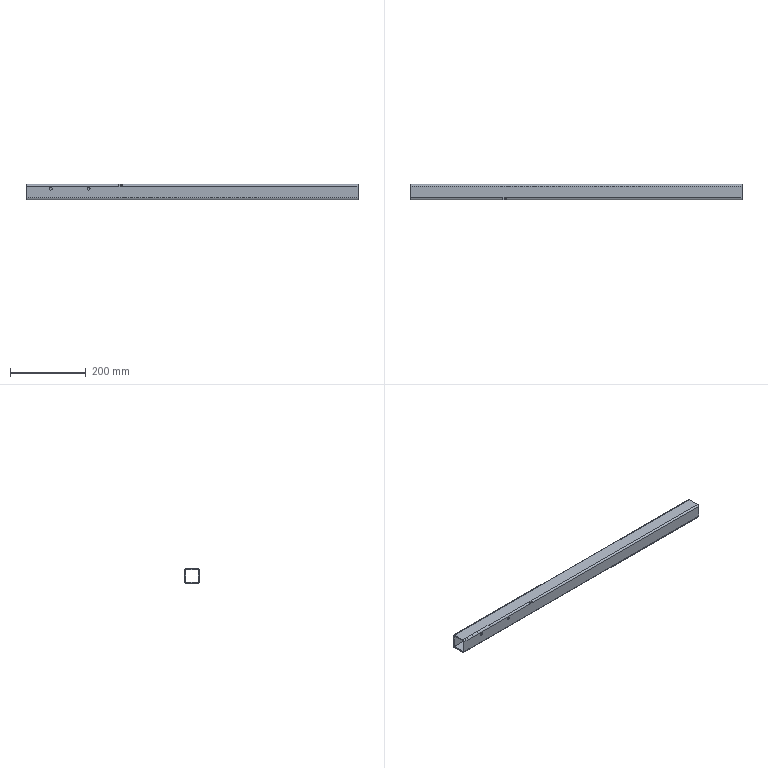Part | 1 solid | 23 faces | box 876 x 40 x 40 mm | volume 373261 mm3 | plane 14 | cylinder 9 | commonest cylinder face diameters 9 x5 8 x4
STEP:
#1=CARTESIAN_POINT('',(-373.,493.,624.88));
#2=VERTEX_POINT('',#1);
#3=CARTESIAN_POINT('',(-373.,493.,632.88));
#4=VERTEX_POINT('',#3);
#5=CARTESIAN_POINT('',(-373.,493.,628.88));
#6=DIRECTION('',(0.,1.,0.));
#7=DIRECTION('',(0.,0.,1.));
#8=AXIS2_PLACEMENT_3D('',#5,#6,#7);
#9=CIRCLE('',#8,4.);
#10=EDGE_CURVE('',#2,#4,#9,.T.);
#11=ORIENTED_EDGE('',*,*,#10,.T.);
#12=CARTESIAN_POINT('',(-373.,490.,632.88));
#13=VERTEX_POINT('',#12);
#14=CARTESIAN_POINT('',(-373.,490.,632.88));
#15=DIRECTION('',(0.,-1.,0.));
#16=VECTOR('',#15,1000.);
#17=LINE('',#14,#16);
#18=EDGE_CURVE('',#4,#13,#17,.T.);
#19=ORIENTED_EDGE('',*,*,#18,.T.);
#20=CARTESIAN_POINT('',(-373.,490.,624.88));
#21=VERTEX_POINT('',#20);
#22=CARTESIAN_POINT('',(-373.,490.,628.88));
#23=DIRECTION('',(0.,-1.,0.));
#24=DIRECTION('',(0.,0.,-1.));
#25=AXIS2_PLACEMENT_3D('',#22,#23,#24);
#26=CIRCLE('',#25,4.);
#27=EDGE_CURVE('',#13,#21,#26,.T.);
#28=ORIENTED_EDGE('',*,*,#27,.T.);
#29=CARTESIAN_POINT('',(-373.,490.,624.88));
#30=DIRECTION('',(0.,-1.,0.));
#31=VECTOR('',#30,1000.);
#32=LINE('',#29,#31);
#33=EDGE_CURVE('',#2,#21,#32,.T.);
#34=ORIENTED_EDGE('',*,*,#33,.F.);
#35=EDGE_LOOP('',(#11,#19,#28,#34));
#36=FACE_OUTER_BOUND('',#35,.T.);
#37=CARTESIAN_POINT('',(-373.,490.,628.88));
#38=DIRECTION('',(0.,-1.,0.));
#39=DIRECTION('',(0.,0.,-1.));
#40=AXIS2_PLACEMENT_3D('',#37,#38,#39);
#41=CYLINDRICAL_SURFACE('',#40,4.);
#42=ADVANCED_FACE('',(#36),#41,.F.);
#43=CARTESIAN_POINT('',(-473.,493.,624.88));
#44=VERTEX_POINT('',#43);
#45=CARTESIAN_POINT('',(-473.,493.,632.88));
#46=VERTEX_POINT('',#45);
#47=CARTESIAN_POINT('',(-473.,493.,628.88));
#48=DIRECTION('',(0.,1.,0.));
#49=DIRECTION('',(0.,0.,1.));
#50=AXIS2_PLACEMENT_3D('',#47,#48,#49);
#51=CIRCLE('',#50,4.);
#52=EDGE_CURVE('',#44,#46,#51,.T.);
#53=ORIENTED_EDGE('',*,*,#52,.T.);
#54=CARTESIAN_POINT('',(-473.,490.,632.88));
#55=VERTEX_POINT('',#54);
#56=CARTESIAN_POINT('',(-473.,490.,632.88));
#57=DIRECTION('',(0.,-1.,0.));
#58=VECTOR('',#57,1000.);
#59=LINE('',#56,#58);
#60=EDGE_CURVE('',#46,#55,#59,.T.);
#61=ORIENTED_EDGE('',*,*,#60,.T.);
#62=CARTESIAN_POINT('',(-473.,490.,624.88));
#63=VERTEX_POINT('',#62);
#64=CARTESIAN_POINT('',(-473.,490.,628.88));
#65=DIRECTION('',(0.,-1.,0.));
#66=DIRECTION('',(0.,0.,-1.));
#67=AXIS2_PLACEMENT_3D('',#64,#65,#66);
#68=CIRCLE('',#67,4.);
#69=EDGE_CURVE('',#55,#63,#68,.T.);
#70=ORIENTED_EDGE('',*,*,#69,.T.);
#71=CARTESIAN_POINT('',(-473.,490.,624.88));
#72=DIRECTION('',(0.,-1.,0.));
#73=VECTOR('',#72,1000.);
#74=LINE('',#71,#73);
#75=EDGE_CURVE('',#44,#63,#74,.T.);
#76=ORIENTED_EDGE('',*,*,#75,.F.);
#77=EDGE_LOOP('',(#53,#61,#70,#76));
#78=FACE_OUTER_BOUND('',#77,.T.);
#79=CARTESIAN_POINT('',(-473.,490.,628.88));
#80=DIRECTION('',(0.,-1.,0.));
#81=DIRECTION('',(0.,0.,-1.));
#82=AXIS2_PLACEMENT_3D('',#79,#80,#81);
#83=CYLINDRICAL_SURFACE('',#82,4.);
#84=ADVANCED_FACE('',(#78),#83,.F.);
#85=CARTESIAN_POINT('',(338.,525.5,640.));
#86=VERTEX_POINT('',#85);
#87=CARTESIAN_POINT('',(338.,494.5,640.));
#88=VERTEX_POINT('',#87);
#89=CARTESIAN_POINT('',(338.,530.,640.));
#90=DIRECTION('',(0.,-1.,0.));
#91=VECTOR('',#90,1000.);
#92=LINE('',#89,#91);
#93=EDGE_CURVE('',#86,#88,#92,.T.);
#94=ORIENTED_EDGE('',*,*,#93,.T.);
#95=CARTESIAN_POINT('',(338.,490.,635.5));
#96=VERTEX_POINT('',#95);
#97=CARTESIAN_POINT('',(338.,494.5,635.5));
#98=DIRECTION('',(1.,0.,0.));
#99=DIRECTION('',(0.,0.,1.));
#100=AXIS2_PLACEMENT_3D('',#97,#98,#99);
#101=CIRCLE('',#100,4.5);
#102=EDGE_CURVE('',#88,#96,#101,.T.);
#103=ORIENTED_EDGE('',*,*,#102,.T.);
#104=CARTESIAN_POINT('',(338.,490.,604.5));
#105=VERTEX_POINT('',#104);
#106=CARTESIAN_POINT('',(338.,490.,640.));
#107=DIRECTION('',(0.,0.,-1.));
#108=VECTOR('',#107,1000.);
#109=LINE('',#106,#108);
#110=EDGE_CURVE('',#96,#105,#109,.T.);
#111=ORIENTED_EDGE('',*,*,#110,.T.);
#112=CARTESIAN_POINT('',(338.,494.5,600.));
#113=VERTEX_POINT('',#112);
#114=CARTESIAN_POINT('',(338.,494.5,604.5));
#115=DIRECTION('',(1.,0.,0.));
#116=DIRECTION('',(0.,0.,1.));
#117=AXIS2_PLACEMENT_3D('',#114,#115,#116);
#118=CIRCLE('',#117,4.5);
#119=EDGE_CURVE('',#105,#113,#118,.T.);
#120=ORIENTED_EDGE('',*,*,#119,.T.);
#121=CARTESIAN_POINT('',(338.,525.5,600.));
#122=VERTEX_POINT('',#121);
#123=CARTESIAN_POINT('',(338.,490.,600.));
#124=DIRECTION('',(0.,-1.,0.));
#125=VECTOR('',#124,1000.);
#126=LINE('',#123,#125);
#127=EDGE_CURVE('',#122,#113,#126,.T.);
#128=ORIENTED_EDGE('',*,*,#127,.F.);
#129=CARTESIAN_POINT('',(338.,530.,604.5));
#130=VERTEX_POINT('',#129);
#131=CARTESIAN_POINT('',(338.,525.5,604.5));
#132=DIRECTION('',(1.,0.,0.));
#133=DIRECTION('',(0.,0.,1.));
#134=AXIS2_PLACEMENT_3D('',#131,#132,#133);
#135=CIRCLE('',#134,4.5);
#136=EDGE_CURVE('',#122,#130,#135,.T.);
#137=ORIENTED_EDGE('',*,*,#136,.T.);
#138=CARTESIAN_POINT('',(338.,530.,635.5));
#139=VERTEX_POINT('',#138);
#140=CARTESIAN_POINT('',(338.,530.,-260.));
#141=DIRECTION('',(0.,0.,-1.));
#142=VECTOR('',#141,1000.);
#143=LINE('',#140,#142);
#144=EDGE_CURVE('',#139,#130,#143,.T.);
#145=ORIENTED_EDGE('',*,*,#144,.F.);
#146=CARTESIAN_POINT('',(338.,525.5,635.5));
#147=DIRECTION('',(1.,0.,0.));
#148=DIRECTION('',(0.,0.,1.));
#149=AXIS2_PLACEMENT_3D('',#146,#147,#148);
#150=CIRCLE('',#149,4.5);
#151=EDGE_CURVE('',#139,#86,#150,.T.);
#152=ORIENTED_EDGE('',*,*,#151,.T.);
#153=EDGE_LOOP('',(#94,#103,#111,#120,#128,#137,#145,#152));
#154=FACE_OUTER_BOUND('',#153,.T.);
#155=CARTESIAN_POINT('',(338.,493.,637.));
#156=VERTEX_POINT('',#155);
#157=CARTESIAN_POINT('',(338.,493.,603.));
#158=VERTEX_POINT('',#157);
#159=CARTESIAN_POINT('',(338.,493.,-260.));
#160=DIRECTION('',(0.,0.,-1.));
#161=VECTOR('',#160,1000.);
#162=LINE('',#159,#161);
#163=EDGE_CURVE('',#156,#158,#162,.T.);
#164=ORIENTED_EDGE('',*,*,#163,.F.);
#165=CARTESIAN_POINT('',(338.,527.,637.));
#166=VERTEX_POINT('',#165);
#167=CARTESIAN_POINT('',(338.,490.,637.));
#168=DIRECTION('',(0.,-1.,0.));
#169=VECTOR('',#168,1000.);
#170=LINE('',#167,#169);
#171=EDGE_CURVE('',#166,#156,#170,.T.);
#172=ORIENTED_EDGE('',*,*,#171,.F.);
#173=CARTESIAN_POINT('',(338.,527.,603.));
#174=VERTEX_POINT('',#173);
#175=CARTESIAN_POINT('',(338.,527.,-260.));
#176=DIRECTION('',(0.,0.,1.));
#177=VECTOR('',#176,1000.);
#178=LINE('',#175,#177);
#179=EDGE_CURVE('',#174,#166,#178,.T.);
#180=ORIENTED_EDGE('',*,*,#179,.F.);
#181=CARTESIAN_POINT('',(338.,490.,603.));
#182=DIRECTION('',(0.,1.,0.));
#183=VECTOR('',#182,1000.);
#184=LINE('',#181,#183);
#185=EDGE_CURVE('',#158,#174,#184,.T.);
#186=ORIENTED_EDGE('',*,*,#185,.F.);
#187=EDGE_LOOP('',(#164,#172,#180,#186));
#188=FACE_BOUND('',#187,.T.);
#189=CARTESIAN_POINT('',(338.,490.,-260.));
#190=DIRECTION('',(-1.,0.,0.));
#191=DIRECTION('',(0.,0.,1.));
#192=AXIS2_PLACEMENT_3D('',#189,#190,#191);
#193=PLANE('',#192);
#194=ADVANCED_FACE('',(#154,#188),#193,.F.);
#195=CARTESIAN_POINT('',(-538.,494.5,640.));
#196=VERTEX_POINT('',#195);
#197=CARTESIAN_POINT('',(-538.,525.5,640.));
#198=VERTEX_POINT('',#197);
#199=CARTESIAN_POINT('',(-538.,530.,640.));
#200=DIRECTION('',(0.,1.,0.));
#201=VECTOR('',#200,1000.);
#202=LINE('',#199,#201);
#203=EDGE_CURVE('',#196,#198,#202,.T.);
#204=ORIENTED_EDGE('',*,*,#203,.T.);
#205=CARTESIAN_POINT('',(-538.,530.,635.5));
#206=VERTEX_POINT('',#205);
#207=CARTESIAN_POINT('',(-538.,525.5,635.5));
#208=DIRECTION('',(-1.,0.,0.));
#209=DIRECTION('',(0.,0.,-1.));
#210=AXIS2_PLACEMENT_3D('',#207,#208,#209);
#211=CIRCLE('',#210,4.5);
#212=EDGE_CURVE('',#198,#206,#211,.T.);
#213=ORIENTED_EDGE('',*,*,#212,.T.);
#214=CARTESIAN_POINT('',(-538.,530.,604.5));
#215=VERTEX_POINT('',#214);
#216=CARTESIAN_POINT('',(-538.,530.,640.));
#217=DIRECTION('',(0.,0.,1.));
#218=VECTOR('',#217,1000.);
#219=LINE('',#216,#218);
#220=EDGE_CURVE('',#215,#206,#219,.T.);
#221=ORIENTED_EDGE('',*,*,#220,.F.);
#222=CARTESIAN_POINT('',(-538.,525.5,600.));
#223=VERTEX_POINT('',#222);
#224=CARTESIAN_POINT('',(-538.,525.5,604.5));
#225=DIRECTION('',(-1.,0.,0.));
#226=DIRECTION('',(0.,0.,-1.));
#227=AXIS2_PLACEMENT_3D('',#224,#225,#226);
#228=CIRCLE('',#227,4.5);
#229=EDGE_CURVE('',#215,#223,#228,.T.);
#230=ORIENTED_EDGE('',*,*,#229,.T.);
#231=CARTESIAN_POINT('',(-538.,494.5,600.));
#232=VERTEX_POINT('',#231);
#233=CARTESIAN_POINT('',(-538.,490.,600.));
#234=DIRECTION('',(0.,1.,0.));
#235=VECTOR('',#234,1000.);
#236=LINE('',#233,#235);
#237=EDGE_CURVE('',#232,#223,#236,.T.);
#238=ORIENTED_EDGE('',*,*,#237,.F.);
#239=CARTESIAN_POINT('',(-538.,490.,604.5));
#240=VERTEX_POINT('',#239);
#241=CARTESIAN_POINT('',(-538.,494.5,604.5));
#242=DIRECTION('',(-1.,0.,0.));
#243=DIRECTION('',(0.,0.,-1.));
#244=AXIS2_PLACEMENT_3D('',#241,#242,#243);
#245=CIRCLE('',#244,4.5);
#246=EDGE_CURVE('',#232,#240,#245,.T.);
#247=ORIENTED_EDGE('',*,*,#246,.T.);
#248=CARTESIAN_POINT('',(-538.,490.,635.5));
#249=VERTEX_POINT('',#248);
#250=CARTESIAN_POINT('',(-538.,490.,640.));
#251=DIRECTION('',(0.,0.,-1.));
#252=VECTOR('',#251,1000.);
#253=LINE('',#250,#252);
#254=EDGE_CURVE('',#249,#240,#253,.T.);
#255=ORIENTED_EDGE('',*,*,#254,.F.);
#256=CARTESIAN_POINT('',(-538.,494.5,635.5));
#257=DIRECTION('',(-1.,0.,0.));
#258=DIRECTION('',(0.,0.,-1.));
#259=AXIS2_PLACEMENT_3D('',#256,#257,#258);
#260=CIRCLE('',#259,4.5);
#261=EDGE_CURVE('',#249,#196,#260,.T.);
#262=ORIENTED_EDGE('',*,*,#261,.T.);
#263=EDGE_LOOP('',(#204,#213,#221,#230,#238,#247,#255,#262));
#264=FACE_OUTER_BOUND('',#263,.T.);
#265=CARTESIAN_POINT('',(-538.,527.,637.));
#266=VERTEX_POINT('',#265);
#267=CARTESIAN_POINT('',(-538.,527.,603.));
#268=VERTEX_POINT('',#267);
#269=CARTESIAN_POINT('',(-538.,527.,640.));
#270=DIRECTION('',(0.,0.,-1.));
#271=VECTOR('',#270,1000.);
#272=LINE('',#269,#271);
#273=EDGE_CURVE('',#266,#268,#272,.T.);
#274=ORIENTED_EDGE('',*,*,#273,.F.);
#275=CARTESIAN_POINT('',(-538.,493.,637.));
#276=VERTEX_POINT('',#275);
#277=CARTESIAN_POINT('',(-538.,490.,637.));
#278=DIRECTION('',(0.,1.,0.));
#279=VECTOR('',#278,1000.);
#280=LINE('',#277,#279);
#281=EDGE_CURVE('',#276,#266,#280,.T.);
#282=ORIENTED_EDGE('',*,*,#281,.F.);
#283=CARTESIAN_POINT('',(-538.,493.,603.));
#284=VERTEX_POINT('',#283);
#285=CARTESIAN_POINT('',(-538.,493.,640.));
#286=DIRECTION('',(0.,0.,1.));
#287=VECTOR('',#286,1000.);
#288=LINE('',#285,#287);
#289=EDGE_CURVE('',#284,#276,#288,.T.);
#290=ORIENTED_EDGE('',*,*,#289,.F.);
#291=CARTESIAN_POINT('',(-538.,490.,603.));
#292=DIRECTION('',(0.,-1.,0.));
#293=VECTOR('',#292,1000.);
#294=LINE('',#291,#293);
#295=EDGE_CURVE('',#268,#284,#294,.T.);
#296=ORIENTED_EDGE('',*,*,#295,.F.);
#297=EDGE_LOOP('',(#274,#282,#290,#296));
#298=FACE_BOUND('',#297,.T.);
#299=CARTESIAN_POINT('',(-538.,490.,640.));
#300=DIRECTION('',(1.,0.,0.));
#301=DIRECTION('',(0.,0.,-1.));
#302=AXIS2_PLACEMENT_3D('',#299,#300,#301);
#303=PLANE('',#302);
#304=ADVANCED_FACE('',(#264,#298),#303,.F.);
#305=CARTESIAN_POINT('',(-293.2,494.5,640.));
#306=VERTEX_POINT('',#305);
#307=CARTESIAN_POINT('',(-293.2,490.,635.5));
#308=VERTEX_POINT('',#307);
#309=CARTESIAN_POINT('',(-293.2,494.5,635.5));
#310=DIRECTION('',(1.,0.,0.));
#311=DIRECTION('',(0.,0.,1.));
#312=AXIS2_PLACEMENT_3D('',#309,#310,#311);
#313=CIRCLE('',#312,4.5);
#314=EDGE_CURVE('',#306,#308,#313,.T.);
#315=ORIENTED_EDGE('',*,*,#314,.F.);
#316=CARTESIAN_POINT('',(160.,494.5,640.));
#317=DIRECTION('',(1.,0.,0.));
#318=VECTOR('',#317,1000.);
#319=LINE('',#316,#318);
#320=EDGE_CURVE('',#196,#306,#319,.T.);
#321=ORIENTED_EDGE('',*,*,#320,.F.);
#322=ORIENTED_EDGE('',*,*,#261,.F.);
#323=CARTESIAN_POINT('',(200.002,490.,635.5));
#324=DIRECTION('',(-1.,0.,0.));
#325=VECTOR('',#324,1000.);
#326=LINE('',#323,#325);
#327=EDGE_CURVE('',#308,#249,#326,.T.);
#328=ORIENTED_EDGE('',*,*,#327,.F.);
#329=EDGE_LOOP('',(#315,#321,#322,#328));
#330=FACE_OUTER_BOUND('',#329,.T.);
#331=CARTESIAN_POINT('',(200.002,494.5,635.5));
#332=DIRECTION('',(-1.,0.,0.));
#333=DIRECTION('',(0.,0.,1.));
#334=AXIS2_PLACEMENT_3D('',#331,#332,#333);
#335=CYLINDRICAL_SURFACE('',#334,4.5);
#336=ADVANCED_FACE('',(#330),#335,.T.);
#337=CARTESIAN_POINT('',(-373.,490.,628.88));
#338=DIRECTION('',(0.,-1.,0.));
#339=DIRECTION('',(0.,0.,-1.));
#340=AXIS2_PLACEMENT_3D('',#337,#338,#339);
#341=CIRCLE('',#340,4.);
#342=EDGE_CURVE('',#21,#13,#341,.T.);
#343=ORIENTED_EDGE('',*,*,#342,.F.);
#344=ORIENTED_EDGE('',*,*,#27,.F.);
#345=EDGE_LOOP('',(#343,#344));
#346=FACE_BOUND('',#345,.T.);
#347=CARTESIAN_POINT('',(-473.,490.,628.88));
#348=DIRECTION('',(0.,-1.,0.));
#349=DIRECTION('',(0.,0.,-1.));
#350=AXIS2_PLACEMENT_3D('',#347,#348,#349);
#351=CIRCLE('',#350,4.);
#352=EDGE_CURVE('',#63,#55,#351,.T.);
#353=ORIENTED_EDGE('',*,*,#352,.F.);
#354=ORIENTED_EDGE('',*,*,#69,.F.);
#355=EDGE_LOOP('',(#353,#354));
#356=FACE_BOUND('',#355,.T.);
#357=CARTESIAN_POINT('',(-293.2,490.,635.3));
#358=VERTEX_POINT('',#357);
#359=CARTESIAN_POINT('',(-282.8,490.,635.3));
#360=VERTEX_POINT('',#359);
#361=CARTESIAN_POINT('',(-293.2,490.,635.3));
#362=DIRECTION('',(1.,0.,0.));
#363=VECTOR('',#362,1000.);
#364=LINE('',#361,#363);
#365=EDGE_CURVE('',#358,#360,#364,.T.);
#366=ORIENTED_EDGE('',*,*,#365,.F.);
#367=CARTESIAN_POINT('',(-293.2,490.,635.3));
#368=DIRECTION('',(0.,0.,1.));
#369=VECTOR('',#368,1000.);
#370=LINE('',#367,#369);
#371=EDGE_CURVE('',#358,#308,#370,.T.);
#372=ORIENTED_EDGE('',*,*,#371,.T.);
#373=ORIENTED_EDGE('',*,*,#327,.T.);
#374=ORIENTED_EDGE('',*,*,#254,.T.);
#375=CARTESIAN_POINT('',(338.,490.,604.5));
#376=DIRECTION('',(1.,0.,0.));
#377=VECTOR('',#376,1000.);
#378=LINE('',#375,#377);
#379=EDGE_CURVE('',#240,#105,#378,.T.);
#380=ORIENTED_EDGE('',*,*,#379,.T.);
#381=ORIENTED_EDGE('',*,*,#110,.F.);
#382=CARTESIAN_POINT('',(-282.8,490.,635.5));
#383=VERTEX_POINT('',#382);
#384=CARTESIAN_POINT('',(200.002,490.,635.5));
#385=DIRECTION('',(-1.,0.,0.));
#386=VECTOR('',#385,1000.);
#387=LINE('',#384,#386);
#388=EDGE_CURVE('',#96,#383,#387,.T.);
#389=ORIENTED_EDGE('',*,*,#388,.T.);
#390=CARTESIAN_POINT('',(-282.8,490.,635.3));
#391=DIRECTION('',(0.,0.,1.));
#392=VECTOR('',#391,1000.);
#393=LINE('',#390,#392);
#394=EDGE_CURVE('',#360,#383,#393,.T.);
#395=ORIENTED_EDGE('',*,*,#394,.F.);
#396=EDGE_LOOP('',(#366,#372,#373,#374,#380,#381,#389,#395));
#397=FACE_OUTER_BOUND('',#396,.T.);
#398=CARTESIAN_POINT('',(200.002,490.,640.));
#399=DIRECTION('',(0.,1.,0.));
#400=DIRECTION('',(0.,0.,1.));
#401=AXIS2_PLACEMENT_3D('',#398,#399,#400);
#402=PLANE('',#401);
#403=ADVANCED_FACE('',(#346,#356,#397),#402,.F.);
#404=ORIENTED_EDGE('',*,*,#320,.T.);
#405=CARTESIAN_POINT('',(-293.2,494.7,640.));
#406=VERTEX_POINT('',#405);
#407=CARTESIAN_POINT('',(-293.2,494.7,640.));
#408=DIRECTION('',(0.,-1.,0.));
#409=VECTOR('',#408,1000.);
#410=LINE('',#407,#409);
#411=EDGE_CURVE('',#406,#306,#410,.T.);
#412=ORIENTED_EDGE('',*,*,#411,.F.);
#413=CARTESIAN_POINT('',(-282.8,494.7,640.));
#414=VERTEX_POINT('',#413);
#415=CARTESIAN_POINT('',(-282.8,494.7,640.));
#416=DIRECTION('',(-1.,0.,0.));
#417=VECTOR('',#416,1000.);
#418=LINE('',#415,#417);
#419=EDGE_CURVE('',#414,#406,#418,.T.);
#420=ORIENTED_EDGE('',*,*,#419,.F.);
#421=CARTESIAN_POINT('',(-282.8,494.5,640.));
#422=VERTEX_POINT('',#421);
#423=CARTESIAN_POINT('',(-282.8,490.,640.));
#424=DIRECTION('',(0.,1.,0.));
#425=VECTOR('',#424,1000.);
#426=LINE('',#423,#425);
#427=EDGE_CURVE('',#422,#414,#426,.T.);
#428=ORIENTED_EDGE('',*,*,#427,.F.);
#429=CARTESIAN_POINT('',(160.,494.5,640.));
#430=DIRECTION('',(1.,0.,0.));
#431=VECTOR('',#430,1000.);
#432=LINE('',#429,#431);
#433=EDGE_CURVE('',#422,#88,#432,.T.);
#434=ORIENTED_EDGE('',*,*,#433,.T.);
#435=ORIENTED_EDGE('',*,*,#93,.F.);
#436=CARTESIAN_POINT('',(160.,525.5,640.));
#437=DIRECTION('',(-1.,0.,0.));
#438=VECTOR('',#437,1000.);
#439=LINE('',#436,#438);
#440=EDGE_CURVE('',#86,#198,#439,.T.);
#441=ORIENTED_EDGE('',*,*,#440,.T.);
#442=ORIENTED_EDGE('',*,*,#203,.F.);
#443=EDGE_LOOP('',(#404,#412,#420,#428,#434,#435,#441,#442));
#444=FACE_OUTER_BOUND('',#443,.T.);
#445=CARTESIAN_POINT('',(160.,530.,640.));
#446=DIRECTION('',(0.,0.,-1.));
#447=DIRECTION('',(-1.,0.,0.));
#448=AXIS2_PLACEMENT_3D('',#445,#446,#447);
#449=PLANE('',#448);
#450=ADVANCED_FACE('',(#444),#449,.F.);
#451=ORIENTED_EDGE('',*,*,#220,.T.);
#452=CARTESIAN_POINT('',(200.,530.,635.5));
#453=DIRECTION('',(1.,0.,0.));
#454=VECTOR('',#453,1000.);
#455=LINE('',#452,#454);
#456=EDGE_CURVE('',#206,#139,#455,.T.);
#457=ORIENTED_EDGE('',*,*,#456,.T.);
#458=ORIENTED_EDGE('',*,*,#144,.T.);
#459=CARTESIAN_POINT('',(-538.,530.,604.5));
#460=DIRECTION('',(-1.,0.,0.));
#461=VECTOR('',#460,1000.);
#462=LINE('',#459,#461);
#463=EDGE_CURVE('',#130,#215,#462,.T.);
#464=ORIENTED_EDGE('',*,*,#463,.T.);
#465=EDGE_LOOP('',(#451,#457,#458,#464));
#466=FACE_OUTER_BOUND('',#465,.T.);
#467=CARTESIAN_POINT('',(200.,530.,-220.));
#468=DIRECTION('',(0.,-1.,0.));
#469=DIRECTION('',(0.,0.,-1.));
#470=AXIS2_PLACEMENT_3D('',#467,#468,#469);
#471=PLANE('',#470);
#472=ADVANCED_FACE('',(#466),#471,.F.);
#473=ORIENTED_EDGE('',*,*,#179,.T.);
#474=CARTESIAN_POINT('',(160.,527.,637.));
#475=DIRECTION('',(-1.,0.,0.));
#476=VECTOR('',#475,1000.);
#477=LINE('',#474,#476);
#478=EDGE_CURVE('',#166,#266,#477,.T.);
#479=ORIENTED_EDGE('',*,*,#478,.T.);
#480=ORIENTED_EDGE('',*,*,#273,.T.);
#481=CARTESIAN_POINT('',(-360.,527.,603.));
#482=DIRECTION('',(-1.,0.,0.));
#483=VECTOR('',#482,1000.);
#484=LINE('',#481,#483);
#485=EDGE_CURVE('',#174,#268,#484,.T.);
#486=ORIENTED_EDGE('',*,*,#485,.F.);
#487=EDGE_LOOP('',(#473,#479,#480,#486));
#488=FACE_OUTER_BOUND('',#487,.T.);
#489=CARTESIAN_POINT('',(-360.,527.,-330.));
#490=DIRECTION('',(0.,-1.,0.));
#491=DIRECTION('',(0.,0.,-1.));
#492=AXIS2_PLACEMENT_3D('',#489,#490,#491);
#493=PLANE('',#492);
#494=ADVANCED_FACE('',(#488),#493,.T.);
#495=CARTESIAN_POINT('',(-293.2,493.,637.));
#496=VERTEX_POINT('',#495);
#497=CARTESIAN_POINT('',(-293.2,494.7,637.));
#498=VERTEX_POINT('',#497);
#499=CARTESIAN_POINT('',(-293.2,530.,637.));
#500=DIRECTION('',(0.,1.,0.));
#501=VECTOR('',#500,1000.);
#502=LINE('',#499,#501);
#503=EDGE_CURVE('',#496,#498,#502,.T.);
#504=ORIENTED_EDGE('',*,*,#503,.F.);
#505=CARTESIAN_POINT('',(400.002,493.,637.));
#506=DIRECTION('',(-1.,0.,0.));
#507=VECTOR('',#506,1000.);
#508=LINE('',#505,#507);
#509=EDGE_CURVE('',#496,#276,#508,.T.);
#510=ORIENTED_EDGE('',*,*,#509,.T.);
#511=ORIENTED_EDGE('',*,*,#281,.T.);
#512=ORIENTED_EDGE('',*,*,#478,.F.);
#513=ORIENTED_EDGE('',*,*,#171,.T.);
#514=CARTESIAN_POINT('',(-282.8,493.,637.));
#515=VERTEX_POINT('',#514);
#516=CARTESIAN_POINT('',(400.002,493.,637.));
#517=DIRECTION('',(-1.,0.,0.));
#518=VECTOR('',#517,1000.);
#519=LINE('',#516,#518);
#520=EDGE_CURVE('',#156,#515,#519,.T.);
#521=ORIENTED_EDGE('',*,*,#520,.T.);
#522=CARTESIAN_POINT('',(-282.8,494.7,637.));
#523=VERTEX_POINT('',#522);
#524=CARTESIAN_POINT('',(-282.8,530.,637.));
#525=DIRECTION('',(0.,-1.,0.));
#526=VECTOR('',#525,1000.);
#527=LINE('',#524,#526);
#528=EDGE_CURVE('',#523,#515,#527,.T.);
#529=ORIENTED_EDGE('',*,*,#528,.F.);
#530=CARTESIAN_POINT('',(160.,494.7,637.));
#531=DIRECTION('',(1.,0.,0.));
#532=VECTOR('',#531,1000.);
#533=LINE('',#530,#532);
#534=EDGE_CURVE('',#498,#523,#533,.T.);
#535=ORIENTED_EDGE('',*,*,#534,.F.);
#536=EDGE_LOOP('',(#504,#510,#511,#512,#513,#521,#529,#535));
#537=FACE_OUTER_BOUND('',#536,.T.);
#538=CARTESIAN_POINT('',(160.,530.,637.));
#539=DIRECTION('',(0.,0.,-1.));
#540=DIRECTION('',(-1.,0.,0.));
#541=AXIS2_PLACEMENT_3D('',#538,#539,#540);
#542=PLANE('',#541);
#543=ADVANCED_FACE('',(#537),#542,.T.);
#544=ORIENTED_EDGE('',*,*,#10,.F.);
#545=CARTESIAN_POINT('',(-373.,493.,628.88));
#546=DIRECTION('',(0.,1.,0.));
#547=DIRECTION('',(0.,0.,1.));
#548=AXIS2_PLACEMENT_3D('',#545,#546,#547);
#549=CIRCLE('',#548,4.);
#550=EDGE_CURVE('',#4,#2,#549,.T.);
#551=ORIENTED_EDGE('',*,*,#550,.F.);
#552=EDGE_LOOP('',(#544,#551));
#553=FACE_BOUND('',#552,.T.);
#554=ORIENTED_EDGE('',*,*,#52,.F.);
#555=CARTESIAN_POINT('',(-473.,493.,628.88));
#556=DIRECTION('',(0.,1.,0.));
#557=DIRECTION('',(0.,0.,1.));
#558=AXIS2_PLACEMENT_3D('',#555,#556,#557);
#559=CIRCLE('',#558,4.);
#560=EDGE_CURVE('',#46,#44,#559,.T.);
#561=ORIENTED_EDGE('',*,*,#560,.F.);
#562=EDGE_LOOP('',(#554,#561));
#563=FACE_BOUND('',#562,.T.);
#564=CARTESIAN_POINT('',(-293.2,493.,635.3));
#565=VERTEX_POINT('',#564);
#566=CARTESIAN_POINT('',(-293.2,493.,640.));
#567=DIRECTION('',(0.,0.,1.));
#568=VECTOR('',#567,1000.);
#569=LINE('',#566,#568);
#570=EDGE_CURVE('',#565,#496,#569,.T.);
#571=ORIENTED_EDGE('',*,*,#570,.F.);
#572=CARTESIAN_POINT('',(-282.8,493.,635.3));
#573=VERTEX_POINT('',#572);
#574=CARTESIAN_POINT('',(400.002,493.,635.3));
#575=DIRECTION('',(1.,0.,0.));
#576=VECTOR('',#575,1000.);
#577=LINE('',#574,#576);
#578=EDGE_CURVE('',#565,#573,#577,.T.);
#579=ORIENTED_EDGE('',*,*,#578,.T.);
#580=CARTESIAN_POINT('',(-282.8,493.,640.));
#581=DIRECTION('',(0.,0.,-1.));
#582=VECTOR('',#581,1000.);
#583=LINE('',#580,#582);
#584=EDGE_CURVE('',#515,#573,#583,.T.);
#585=ORIENTED_EDGE('',*,*,#584,.F.);
#586=ORIENTED_EDGE('',*,*,#520,.F.);
#587=ORIENTED_EDGE('',*,*,#163,.T.);
#588=CARTESIAN_POINT('',(400.002,493.,603.));
#589=DIRECTION('',(1.,0.,0.));
#590=VECTOR('',#589,1000.);
#591=LINE('',#588,#590);
#592=EDGE_CURVE('',#284,#158,#591,.T.);
#593=ORIENTED_EDGE('',*,*,#592,.F.);
#594=ORIENTED_EDGE('',*,*,#289,.T.);
#595=ORIENTED_EDGE('',*,*,#509,.F.);
#596=EDGE_LOOP('',(#571,#579,#585,#586,#587,#593,#594,#595));
#597=FACE_OUTER_BOUND('',#596,.T.);
#598=CARTESIAN_POINT('',(400.002,493.,640.));
#599=DIRECTION('',(0.,1.,0.));
#600=DIRECTION('',(0.,0.,1.));
#601=AXIS2_PLACEMENT_3D('',#598,#599,#600);
#602=PLANE('',#601);
#603=ADVANCED_FACE('',(#553,#563,#597),#602,.T.);
#604=ORIENTED_EDGE('',*,*,#295,.T.);
#605=ORIENTED_EDGE('',*,*,#592,.T.);
#606=ORIENTED_EDGE('',*,*,#185,.T.);
#607=ORIENTED_EDGE('',*,*,#485,.T.);
#608=EDGE_LOOP('',(#604,#605,#606,#607));
#609=FACE_OUTER_BOUND('',#608,.T.);
#610=CARTESIAN_POINT('',(160.,530.,603.));
#611=DIRECTION('',(0.,0.,1.));
#612=DIRECTION('',(1.,0.,0.));
#613=AXIS2_PLACEMENT_3D('',#610,#611,#612);
#614=PLANE('',#613);
#615=ADVANCED_FACE('',(#609),#614,.T.);
#616=ORIENTED_EDGE('',*,*,#127,.T.);
#617=CARTESIAN_POINT('',(-538.,494.5,600.));
#618=DIRECTION('',(-1.,0.,0.));
#619=VECTOR('',#618,1000.);
#620=LINE('',#617,#619);
#621=EDGE_CURVE('',#113,#232,#620,.T.);
#622=ORIENTED_EDGE('',*,*,#621,.T.);
#623=ORIENTED_EDGE('',*,*,#237,.T.);
#624=CARTESIAN_POINT('',(338.,525.5,600.));
#625=DIRECTION('',(1.,0.,0.));
#626=VECTOR('',#625,1000.);
#627=LINE('',#624,#626);
#628=EDGE_CURVE('',#223,#122,#627,.T.);
#629=ORIENTED_EDGE('',*,*,#628,.T.);
#630=EDGE_LOOP('',(#616,#622,#623,#629));
#631=FACE_OUTER_BOUND('',#630,.T.);
#632=CARTESIAN_POINT('',(-20.,23.5,600.));
#633=DIRECTION('',(0.,0.,-1.));
#634=DIRECTION('',(-1.,0.,0.));
#635=AXIS2_PLACEMENT_3D('',#632,#633,#634);
#636=PLANE('',#635);
#637=ADVANCED_FACE('',(#631),#636,.T.);
#638=ORIENTED_EDGE('',*,*,#119,.F.);
#639=ORIENTED_EDGE('',*,*,#379,.F.);
#640=ORIENTED_EDGE('',*,*,#246,.F.);
#641=ORIENTED_EDGE('',*,*,#621,.F.);
#642=EDGE_LOOP('',(#638,#639,#640,#641));
#643=FACE_OUTER_BOUND('',#642,.T.);
#644=CARTESIAN_POINT('',(-20.,494.5,604.5));
#645=DIRECTION('',(1.,0.,0.));
#646=DIRECTION('',(0.,0.,-1.));
#647=AXIS2_PLACEMENT_3D('',#644,#645,#646);
#648=CYLINDRICAL_SURFACE('',#647,4.5);
#649=ADVANCED_FACE('',(#643),#648,.T.);
#650=CARTESIAN_POINT('',(-282.8,494.5,635.5));
#651=DIRECTION('',(-1.,0.,0.));
#652=DIRECTION('',(0.,0.,-1.));
#653=AXIS2_PLACEMENT_3D('',#650,#651,#652);
#654=CIRCLE('',#653,4.5);
#655=EDGE_CURVE('',#383,#422,#654,.T.);
#656=ORIENTED_EDGE('',*,*,#655,.F.);
#657=ORIENTED_EDGE('',*,*,#388,.F.);
#658=ORIENTED_EDGE('',*,*,#102,.F.);
#659=ORIENTED_EDGE('',*,*,#433,.F.);
#660=EDGE_LOOP('',(#656,#657,#658,#659));
#661=FACE_OUTER_BOUND('',#660,.T.);
#662=CARTESIAN_POINT('',(200.002,494.5,635.5));
#663=DIRECTION('',(-1.,0.,0.));
#664=DIRECTION('',(0.,0.,1.));
#665=AXIS2_PLACEMENT_3D('',#662,#663,#664);
#666=CYLINDRICAL_SURFACE('',#665,4.5);
#667=ADVANCED_FACE('',(#661),#666,.T.);
#668=ORIENTED_EDGE('',*,*,#212,.F.);
#669=ORIENTED_EDGE('',*,*,#440,.F.);
#670=ORIENTED_EDGE('',*,*,#151,.F.);
#671=ORIENTED_EDGE('',*,*,#456,.F.);
#672=EDGE_LOOP('',(#668,#669,#670,#671));
#673=FACE_OUTER_BOUND('',#672,.T.);
#674=CARTESIAN_POINT('',(200.,525.5,635.5));
#675=DIRECTION('',(1.,0.,0.));
#676=DIRECTION('',(0.,0.,-1.));
#677=AXIS2_PLACEMENT_3D('',#674,#675,#676);
#678=CYLINDRICAL_SURFACE('',#677,4.5);
#679=ADVANCED_FACE('',(#673),#678,.T.);
#680=ORIENTED_EDGE('',*,*,#229,.F.);
#681=ORIENTED_EDGE('',*,*,#463,.F.);
#682=ORIENTED_EDGE('',*,*,#136,.F.);
#683=ORIENTED_EDGE('',*,*,#628,.F.);
#684=EDGE_LOOP('',(#680,#681,#682,#683));
#685=FACE_OUTER_BOUND('',#684,.T.);
#686=CARTESIAN_POINT('',(-20.,525.5,604.5));
#687=DIRECTION('',(-1.,0.,0.));
#688=DIRECTION('',(0.,0.,1.));
#689=AXIS2_PLACEMENT_3D('',#686,#687,#688);
#690=CYLINDRICAL_SURFACE('',#689,4.5);
#691=ADVANCED_FACE('',(#685),#690,.T.);
#692=ORIENTED_EDGE('',*,*,#570,.T.);
#693=ORIENTED_EDGE('',*,*,#503,.T.);
#694=CARTESIAN_POINT('',(-293.2,494.7,635.3));
#695=DIRECTION('',(0.,0.,1.));
#696=VECTOR('',#695,1000.);
#697=LINE('',#694,#696);
#698=EDGE_CURVE('',#498,#406,#697,.T.);
#699=ORIENTED_EDGE('',*,*,#698,.T.);
#700=ORIENTED_EDGE('',*,*,#411,.T.);
#701=ORIENTED_EDGE('',*,*,#314,.T.);
#702=ORIENTED_EDGE('',*,*,#371,.F.);
#703=CARTESIAN_POINT('',(-293.2,494.7,635.3));
#704=DIRECTION('',(0.,-1.,0.));
#705=VECTOR('',#704,1000.);
#706=LINE('',#703,#705);
#707=EDGE_CURVE('',#565,#358,#706,.T.);
#708=ORIENTED_EDGE('',*,*,#707,.F.);
#709=EDGE_LOOP('',(#692,#693,#699,#700,#701,#702,#708));
#710=FACE_OUTER_BOUND('',#709,.T.);
#711=CARTESIAN_POINT('',(-293.2,494.7,635.3));
#712=DIRECTION('',(-1.,0.,0.));
#713=DIRECTION('',(0.,0.,1.));
#714=AXIS2_PLACEMENT_3D('',#711,#712,#713);
#715=PLANE('',#714);
#716=ADVANCED_FACE('',(#710),#715,.F.);
#717=ORIENTED_EDGE('',*,*,#534,.T.);
#718=CARTESIAN_POINT('',(-282.8,494.7,635.3));
#719=DIRECTION('',(0.,0.,1.));
#720=VECTOR('',#719,1000.);
#721=LINE('',#718,#720);
#722=EDGE_CURVE('',#523,#414,#721,.T.);
#723=ORIENTED_EDGE('',*,*,#722,.T.);
#724=ORIENTED_EDGE('',*,*,#419,.T.);
#725=ORIENTED_EDGE('',*,*,#698,.F.);
#726=EDGE_LOOP('',(#717,#723,#724,#725));
#727=FACE_OUTER_BOUND('',#726,.T.);
#728=CARTESIAN_POINT('',(-282.8,494.7,635.3));
#729=DIRECTION('',(0.,1.,0.));
#730=DIRECTION('',(0.,0.,1.));
#731=AXIS2_PLACEMENT_3D('',#728,#729,#730);
#732=PLANE('',#731);
#733=ADVANCED_FACE('',(#727),#732,.F.);
#734=ORIENTED_EDGE('',*,*,#584,.T.);
#735=CARTESIAN_POINT('',(-282.8,490.,635.3));
#736=DIRECTION('',(0.,1.,0.));
#737=VECTOR('',#736,1000.);
#738=LINE('',#735,#737);
#739=EDGE_CURVE('',#360,#573,#738,.T.);
#740=ORIENTED_EDGE('',*,*,#739,.F.);
#741=ORIENTED_EDGE('',*,*,#394,.T.);
#742=ORIENTED_EDGE('',*,*,#655,.T.);
#743=ORIENTED_EDGE('',*,*,#427,.T.);
#744=ORIENTED_EDGE('',*,*,#722,.F.);
#745=ORIENTED_EDGE('',*,*,#528,.T.);
#746=EDGE_LOOP('',(#734,#740,#741,#742,#743,#744,#745));
#747=FACE_OUTER_BOUND('',#746,.T.);
#748=CARTESIAN_POINT('',(-282.8,490.,635.3));
#749=DIRECTION('',(1.,0.,0.));
#750=DIRECTION('',(0.,0.,-1.));
#751=AXIS2_PLACEMENT_3D('',#748,#749,#750);
#752=PLANE('',#751);
#753=ADVANCED_FACE('',(#747),#752,.F.);
#754=ORIENTED_EDGE('',*,*,#707,.T.);
#755=ORIENTED_EDGE('',*,*,#365,.T.);
#756=ORIENTED_EDGE('',*,*,#739,.T.);
#757=ORIENTED_EDGE('',*,*,#578,.F.);
#758=EDGE_LOOP('',(#754,#755,#756,#757));
#759=FACE_OUTER_BOUND('',#758,.T.);
#760=CARTESIAN_POINT('',(0.,0.,635.3));
#761=DIRECTION('',(0.,0.,1.));
#762=DIRECTION('',(1.,0.,0.));
#763=AXIS2_PLACEMENT_3D('',#760,#761,#762);
#764=PLANE('',#763);
#765=ADVANCED_FACE('',(#759),#764,.T.);
#766=ORIENTED_EDGE('',*,*,#60,.F.);
#767=ORIENTED_EDGE('',*,*,#560,.T.);
#768=ORIENTED_EDGE('',*,*,#75,.T.);
#769=ORIENTED_EDGE('',*,*,#352,.T.);
#770=EDGE_LOOP('',(#766,#767,#768,#769));
#771=FACE_OUTER_BOUND('',#770,.T.);
#772=CARTESIAN_POINT('',(-473.,490.,628.88));
#773=DIRECTION('',(0.,-1.,0.));
#774=DIRECTION('',(0.,0.,-1.));
#775=AXIS2_PLACEMENT_3D('',#772,#773,#774);
#776=CYLINDRICAL_SURFACE('',#775,4.);
#777=ADVANCED_FACE('',(#771),#776,.F.);
#778=ORIENTED_EDGE('',*,*,#18,.F.);
#779=ORIENTED_EDGE('',*,*,#550,.T.);
#780=ORIENTED_EDGE('',*,*,#33,.T.);
#781=ORIENTED_EDGE('',*,*,#342,.T.);
#782=EDGE_LOOP('',(#778,#779,#780,#781));
#783=FACE_OUTER_BOUND('',#782,.T.);
#784=CARTESIAN_POINT('',(-373.,490.,628.88));
#785=DIRECTION('',(0.,-1.,0.));
#786=DIRECTION('',(0.,0.,-1.));
#787=AXIS2_PLACEMENT_3D('',#784,#785,#786);
#788=CYLINDRICAL_SURFACE('',#787,4.);
#789=ADVANCED_FACE('',(#783),#788,.F.);
#790=CLOSED_SHELL('',(#42,#84,#194,#304,#336,#403,#450,#472,#494,#543,#603,#615,#637,#649,#667,#679,#691,#716,#733,#753,#765,#777,#789));
#791=MANIFOLD_SOLID_BREP('',#790);
#792=CARTESIAN_POINT('',(0.,0.,0.));
#793=DIRECTION('',(0.,0.,1.));
#794=DIRECTION('',(1.,0.,0.));
#795=AXIS2_PLACEMENT_3D('',#792,#793,#794);
#796=(LENGTH_UNIT()NAMED_UNIT(*)SI_UNIT(.MILLI.,.METRE.));
#797=UNCERTAINTY_MEASURE_WITH_UNIT(LENGTH_MEASURE(0.00001),#796,'','');
#798=(NAMED_UNIT(*)PLANE_ANGLE_UNIT()SI_UNIT($,.RADIAN.));
#799=(NAMED_UNIT(*)SI_UNIT($,.STERADIAN.)SOLID_ANGLE_UNIT());
#800=(GEOMETRIC_REPRESENTATION_CONTEXT(3)GLOBAL_UNCERTAINTY_ASSIGNED_CONTEXT((#797))GLOBAL_UNIT_ASSIGNED_CONTEXT((#796,#798,#799))REPRESENTATION_CONTEXT('',''));
#801=ADVANCED_BREP_SHAPE_REPRESENTATION('',(#791,#795),#800);